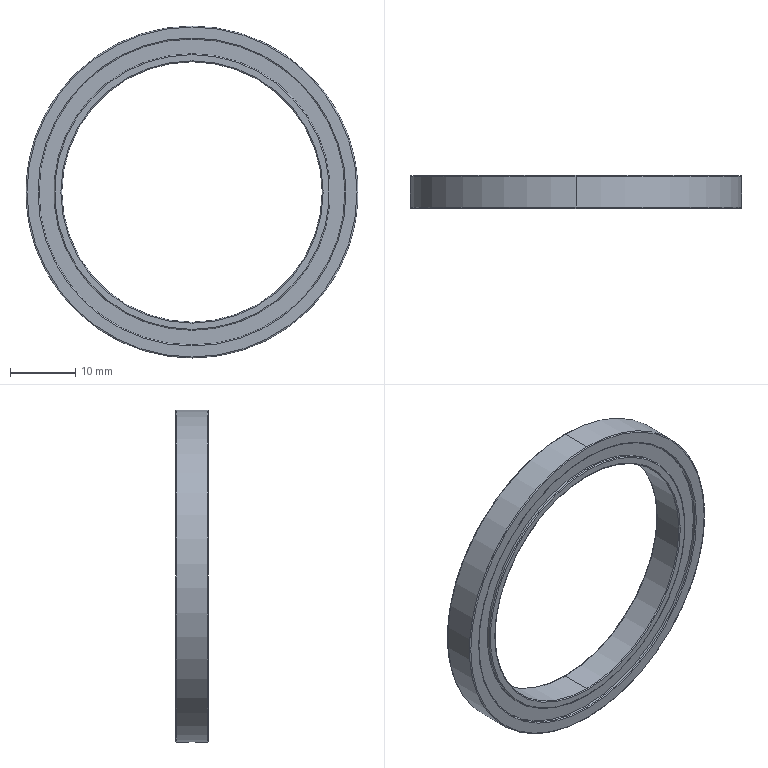Part | SolidWorks | features ICE 3, Extrusion 1, Fillet 1, RefAxis 1, RevCut 1 | 1 solid | 40 faces | box 51 x 5 x 51 mm | volume 3359 mm3 | torus 20 | cylinder 14 | plane 6 | commonest cylinder face diameters 42.5 x4 47 x4 1 x2 40 x2 51 x2
STEP:
#1=CARTESIAN_POINT('',(0.,0.,21.6));
#2=VERTEX_POINT('',#1);
#3=CARTESIAN_POINT('',(0.,0.,23.1));
#4=VERTEX_POINT('',#3);
#5=CARTESIAN_POINT('',(0.,0.,22.35));
#6=DIRECTION('',(-1.,0.,0.));
#7=DIRECTION('',(0.,0.,1.));
#8=AXIS2_PLACEMENT_3D('',#5,#6,#7);
#9=CIRCLE('',#8,0.75);
#10=EDGE_CURVE('',#2,#4,#9,.T.);
#11=ORIENTED_EDGE('',*,*,#10,.T.);
#12=CARTESIAN_POINT('',(0.5,0.,-23.095));
#13=VERTEX_POINT('',#12);
#14=CARTESIAN_POINT('',(0.,0.,0.));
#15=DIRECTION('',(0.,1.,0.));
#16=DIRECTION('',(0.,0.,1.));
#17=AXIS2_PLACEMENT_3D('',#14,#15,#16);
#18=CIRCLE('',#17,23.1);
#19=EDGE_CURVE('',#4,#13,#18,.T.);
#20=ORIENTED_EDGE('',*,*,#19,.T.);
#21=CARTESIAN_POINT('',(0.,-0.5,-22.909));
#22=VERTEX_POINT('',#21);
#23=CARTESIAN_POINT('',(0.5,0.,-23.095));
#24=CARTESIAN_POINT('',(0.5,-0.06758,-23.095));
#25=CARTESIAN_POINT('',(0.4859,-0.1352,-23.085));
#26=CARTESIAN_POINT('',(0.4343,-0.2563,-23.054));
#27=CARTESIAN_POINT('',(0.3972,-0.3102,-23.031));
#28=CARTESIAN_POINT('',(0.3074,-0.3994,-22.985));
#29=CARTESIAN_POINT('',(0.254,-0.4355,-22.96));
#30=CARTESIAN_POINT('',(0.1353,-0.4856,-22.922));
#31=CARTESIAN_POINT('',(0.06827,-0.5,-22.909));
#32=CARTESIAN_POINT('',(0.,-0.5,-22.909));
#33=B_SPLINE_CURVE_WITH_KNOTS('',3,(#23,#24,#25,#26,#27,#28,#29,#30,#31,#32),.UNSPECIFIED.,.F.,.F.,(4,2,2,2,4),(0.002057,0.002259,0.00246,0.002661,0.002863),.UNSPECIFIED.);
#34=EDGE_CURVE('',#13,#22,#33,.T.);
#35=ORIENTED_EDGE('',*,*,#34,.T.);
#36=CARTESIAN_POINT('',(0.,0.,-21.6));
#37=VERTEX_POINT('',#36);
#38=CARTESIAN_POINT('',(0.,0.,-22.35));
#39=DIRECTION('',(1.,0.,0.));
#40=DIRECTION('',(0.,0.,-1.));
#41=AXIS2_PLACEMENT_3D('',#38,#39,#40);
#42=CIRCLE('',#41,0.75);
#43=EDGE_CURVE('',#37,#22,#42,.T.);
#44=ORIENTED_EDGE('',*,*,#43,.F.);
#45=CARTESIAN_POINT('',(0.,0.,0.));
#46=DIRECTION('',(0.,1.,0.));
#47=DIRECTION('',(0.,0.,1.));
#48=AXIS2_PLACEMENT_3D('',#45,#46,#47);
#49=CIRCLE('',#48,21.6);
#50=EDGE_CURVE('',#2,#37,#49,.T.);
#51=ORIENTED_EDGE('',*,*,#50,.F.);
#52=EDGE_LOOP('',(#11,#20,#35,#44,#51));
#53=FACE_OUTER_BOUND('',#52,.T.);
#54=CARTESIAN_POINT('',(0.,0.,0.));
#55=DIRECTION('',(0.,1.,0.));
#56=DIRECTION('',(0.,0.,1.));
#57=AXIS2_PLACEMENT_3D('',#54,#55,#56);
#58=TOROIDAL_SURFACE('',#57,22.35,0.75);
#59=ADVANCED_FACE('',(#53),#58,.F.);
#60=CARTESIAN_POINT('',(-0.5,0.,-23.095));
#61=VERTEX_POINT('',#60);
#62=CARTESIAN_POINT('',(0.,-0.5,-22.909));
#63=CARTESIAN_POINT('',(-0.1367,-0.5,-22.909));
#64=CARTESIAN_POINT('',(-0.2637,-0.4433,-22.962));
#65=CARTESIAN_POINT('',(-0.3982,-0.309,-23.032));
#66=CARTESIAN_POINT('',(-0.4351,-0.2549,-23.054));
#67=CARTESIAN_POINT('',(-0.4859,-0.1348,-23.085));
#68=CARTESIAN_POINT('',(-0.5,-0.06715,-23.095));
#69=CARTESIAN_POINT('',(-0.5,0.,-23.095));
#70=B_SPLINE_CURVE_WITH_KNOTS('',3,(#62,#63,#64,#65,#66,#67,#68,#69),.UNSPECIFIED.,.F.,.F.,(4,2,2,4),(0.002863,0.003266,0.003468,0.003669),.UNSPECIFIED.);
#71=EDGE_CURVE('',#22,#61,#70,.T.);
#72=ORIENTED_EDGE('',*,*,#71,.T.);
#73=CARTESIAN_POINT('',(0.,0.,0.));
#74=DIRECTION('',(0.,1.,0.));
#75=DIRECTION('',(0.,0.,1.));
#76=AXIS2_PLACEMENT_3D('',#73,#74,#75);
#77=CIRCLE('',#76,23.1);
#78=EDGE_CURVE('',#61,#4,#77,.T.);
#79=ORIENTED_EDGE('',*,*,#78,.T.);
#80=ORIENTED_EDGE('',*,*,#10,.F.);
#81=CARTESIAN_POINT('',(0.,0.,0.));
#82=DIRECTION('',(0.,1.,0.));
#83=DIRECTION('',(0.,0.,1.));
#84=AXIS2_PLACEMENT_3D('',#81,#82,#83);
#85=CIRCLE('',#84,21.6);
#86=EDGE_CURVE('',#37,#2,#85,.T.);
#87=ORIENTED_EDGE('',*,*,#86,.F.);
#88=ORIENTED_EDGE('',*,*,#43,.T.);
#89=EDGE_LOOP('',(#72,#79,#80,#87,#88));
#90=FACE_OUTER_BOUND('',#89,.T.);
#91=CARTESIAN_POINT('',(0.,0.,0.));
#92=DIRECTION('',(0.,1.,0.));
#93=DIRECTION('',(0.,0.,1.));
#94=AXIS2_PLACEMENT_3D('',#91,#92,#93);
#95=TOROIDAL_SURFACE('',#94,22.35,0.75);
#96=ADVANCED_FACE('',(#90),#95,.F.);
#97=CARTESIAN_POINT('',(0.,2.5,-23.65));
#98=VERTEX_POINT('',#97);
#99=CARTESIAN_POINT('',(0.,2.5,23.65));
#100=VERTEX_POINT('',#99);
#101=CARTESIAN_POINT('',(0.,2.5,0.));
#102=DIRECTION('',(0.,-1.,0.));
#103=DIRECTION('',(0.,0.,1.));
#104=AXIS2_PLACEMENT_3D('',#101,#102,#103);
#105=CIRCLE('',#104,23.65);
#106=EDGE_CURVE('',#98,#100,#105,.T.);
#107=ORIENTED_EDGE('',*,*,#106,.F.);
#108=CARTESIAN_POINT('',(0.,2.35,-23.5));
#109=VERTEX_POINT('',#108);
#110=CARTESIAN_POINT('',(0.,2.35,-23.65));
#111=DIRECTION('',(1.,0.,0.));
#112=DIRECTION('',(0.,0.,-1.));
#113=AXIS2_PLACEMENT_3D('',#110,#111,#112);
#114=CIRCLE('',#113,0.15);
#115=EDGE_CURVE('',#98,#109,#114,.T.);
#116=ORIENTED_EDGE('',*,*,#115,.T.);
#117=CARTESIAN_POINT('',(0.,2.35,23.5));
#118=VERTEX_POINT('',#117);
#119=CARTESIAN_POINT('',(0.,2.35,0.));
#120=DIRECTION('',(0.,1.,0.));
#121=DIRECTION('',(0.,0.,1.));
#122=AXIS2_PLACEMENT_3D('',#119,#120,#121);
#123=CIRCLE('',#122,23.5);
#124=EDGE_CURVE('',#118,#109,#123,.T.);
#125=ORIENTED_EDGE('',*,*,#124,.F.);
#126=CARTESIAN_POINT('',(0.,2.35,23.65));
#127=DIRECTION('',(-1.,0.,0.));
#128=DIRECTION('',(0.,0.,1.));
#129=AXIS2_PLACEMENT_3D('',#126,#127,#128);
#130=CIRCLE('',#129,0.15);
#131=EDGE_CURVE('',#100,#118,#130,.T.);
#132=ORIENTED_EDGE('',*,*,#131,.F.);
#133=EDGE_LOOP('',(#107,#116,#125,#132));
#134=FACE_OUTER_BOUND('',#133,.T.);
#135=CARTESIAN_POINT('',(0.,2.35,0.));
#136=DIRECTION('',(0.,1.,0.));
#137=DIRECTION('',(0.,0.,1.));
#138=AXIS2_PLACEMENT_3D('',#135,#136,#137);
#139=TOROIDAL_SURFACE('',#138,23.65,0.15);
#140=ADVANCED_FACE('',(#134),#139,.T.);
#141=CARTESIAN_POINT('',(0.,2.35,-25.5));
#142=VERTEX_POINT('',#141);
#143=CARTESIAN_POINT('',(0.,2.35,25.5));
#144=VERTEX_POINT('',#143);
#145=CARTESIAN_POINT('',(0.,2.35,0.));
#146=DIRECTION('',(0.,-1.,0.));
#147=DIRECTION('',(0.,0.,1.));
#148=AXIS2_PLACEMENT_3D('',#145,#146,#147);
#149=CIRCLE('',#148,25.5);
#150=EDGE_CURVE('',#142,#144,#149,.T.);
#151=ORIENTED_EDGE('',*,*,#150,.F.);
#152=CARTESIAN_POINT('',(0.,2.5,-25.35));
#153=VERTEX_POINT('',#152);
#154=CARTESIAN_POINT('',(0.,2.35,-25.35));
#155=DIRECTION('',(1.,0.,0.));
#156=DIRECTION('',(0.,0.,-1.));
#157=AXIS2_PLACEMENT_3D('',#154,#155,#156);
#158=CIRCLE('',#157,0.15);
#159=EDGE_CURVE('',#142,#153,#158,.T.);
#160=ORIENTED_EDGE('',*,*,#159,.T.);
#161=CARTESIAN_POINT('',(0.,2.5,25.35));
#162=VERTEX_POINT('',#161);
#163=CARTESIAN_POINT('',(0.,2.5,0.));
#164=DIRECTION('',(0.,1.,0.));
#165=DIRECTION('',(0.,0.,1.));
#166=AXIS2_PLACEMENT_3D('',#163,#164,#165);
#167=CIRCLE('',#166,25.35);
#168=EDGE_CURVE('',#162,#153,#167,.T.);
#169=ORIENTED_EDGE('',*,*,#168,.F.);
#170=CARTESIAN_POINT('',(0.,2.35,25.35));
#171=DIRECTION('',(-1.,0.,0.));
#172=DIRECTION('',(0.,0.,1.));
#173=AXIS2_PLACEMENT_3D('',#170,#171,#172);
#174=CIRCLE('',#173,0.15);
#175=EDGE_CURVE('',#144,#162,#174,.T.);
#176=ORIENTED_EDGE('',*,*,#175,.F.);
#177=EDGE_LOOP('',(#151,#160,#169,#176));
#178=FACE_OUTER_BOUND('',#177,.T.);
#179=CARTESIAN_POINT('',(0.,2.35,0.));
#180=DIRECTION('',(0.,1.,0.));
#181=DIRECTION('',(0.,0.,1.));
#182=AXIS2_PLACEMENT_3D('',#179,#180,#181);
#183=TOROIDAL_SURFACE('',#182,25.35,0.15);
#184=ADVANCED_FACE('',(#178),#183,.T.);
#185=CARTESIAN_POINT('',(0.,2.5,-20.15));
#186=VERTEX_POINT('',#185);
#187=CARTESIAN_POINT('',(0.,2.5,20.15));
#188=VERTEX_POINT('',#187);
#189=CARTESIAN_POINT('',(0.,2.5,0.));
#190=DIRECTION('',(0.,-1.,0.));
#191=DIRECTION('',(0.,0.,1.));
#192=AXIS2_PLACEMENT_3D('',#189,#190,#191);
#193=CIRCLE('',#192,20.15);
#194=EDGE_CURVE('',#186,#188,#193,.T.);
#195=ORIENTED_EDGE('',*,*,#194,.F.);
#196=CARTESIAN_POINT('',(0.,2.35,-20.));
#197=VERTEX_POINT('',#196);
#198=CARTESIAN_POINT('',(0.,2.35,-20.15));
#199=DIRECTION('',(1.,0.,0.));
#200=DIRECTION('',(0.,0.,-1.));
#201=AXIS2_PLACEMENT_3D('',#198,#199,#200);
#202=CIRCLE('',#201,0.15);
#203=EDGE_CURVE('',#186,#197,#202,.T.);
#204=ORIENTED_EDGE('',*,*,#203,.T.);
#205=CARTESIAN_POINT('',(0.,2.35,20.));
#206=VERTEX_POINT('',#205);
#207=CARTESIAN_POINT('',(0.,2.35,0.));
#208=DIRECTION('',(0.,1.,0.));
#209=DIRECTION('',(0.,0.,1.));
#210=AXIS2_PLACEMENT_3D('',#207,#208,#209);
#211=CIRCLE('',#210,20.);
#212=EDGE_CURVE('',#206,#197,#211,.T.);
#213=ORIENTED_EDGE('',*,*,#212,.F.);
#214=CARTESIAN_POINT('',(0.,2.35,20.15));
#215=DIRECTION('',(-1.,0.,0.));
#216=DIRECTION('',(0.,0.,1.));
#217=AXIS2_PLACEMENT_3D('',#214,#215,#216);
#218=CIRCLE('',#217,0.15);
#219=EDGE_CURVE('',#188,#206,#218,.T.);
#220=ORIENTED_EDGE('',*,*,#219,.F.);
#221=EDGE_LOOP('',(#195,#204,#213,#220));
#222=FACE_OUTER_BOUND('',#221,.T.);
#223=CARTESIAN_POINT('',(0.,2.35,0.));
#224=DIRECTION('',(0.,1.,0.));
#225=DIRECTION('',(0.,0.,1.));
#226=AXIS2_PLACEMENT_3D('',#223,#224,#225);
#227=TOROIDAL_SURFACE('',#226,20.15,0.15);
#228=ADVANCED_FACE('',(#222),#227,.T.);
#229=CARTESIAN_POINT('',(0.,2.35,-21.25));
#230=VERTEX_POINT('',#229);
#231=CARTESIAN_POINT('',(0.,2.35,21.25));
#232=VERTEX_POINT('',#231);
#233=CARTESIAN_POINT('',(0.,2.35,0.));
#234=DIRECTION('',(0.,-1.,0.));
#235=DIRECTION('',(0.,0.,1.));
#236=AXIS2_PLACEMENT_3D('',#233,#234,#235);
#237=CIRCLE('',#236,21.25);
#238=EDGE_CURVE('',#230,#232,#237,.T.);
#239=ORIENTED_EDGE('',*,*,#238,.F.);
#240=CARTESIAN_POINT('',(0.,2.5,-21.1));
#241=VERTEX_POINT('',#240);
#242=CARTESIAN_POINT('',(0.,2.35,-21.1));
#243=DIRECTION('',(1.,0.,0.));
#244=DIRECTION('',(0.,0.,-1.));
#245=AXIS2_PLACEMENT_3D('',#242,#243,#244);
#246=CIRCLE('',#245,0.15);
#247=EDGE_CURVE('',#230,#241,#246,.T.);
#248=ORIENTED_EDGE('',*,*,#247,.T.);
#249=CARTESIAN_POINT('',(0.,2.5,21.1));
#250=VERTEX_POINT('',#249);
#251=CARTESIAN_POINT('',(0.,2.5,0.));
#252=DIRECTION('',(0.,1.,0.));
#253=DIRECTION('',(0.,0.,1.));
#254=AXIS2_PLACEMENT_3D('',#251,#252,#253);
#255=CIRCLE('',#254,21.1);
#256=EDGE_CURVE('',#250,#241,#255,.T.);
#257=ORIENTED_EDGE('',*,*,#256,.F.);
#258=CARTESIAN_POINT('',(0.,2.35,21.1));
#259=DIRECTION('',(-1.,0.,0.));
#260=DIRECTION('',(0.,0.,1.));
#261=AXIS2_PLACEMENT_3D('',#258,#259,#260);
#262=CIRCLE('',#261,0.15);
#263=EDGE_CURVE('',#232,#250,#262,.T.);
#264=ORIENTED_EDGE('',*,*,#263,.F.);
#265=EDGE_LOOP('',(#239,#248,#257,#264));
#266=FACE_OUTER_BOUND('',#265,.T.);
#267=CARTESIAN_POINT('',(0.,2.35,0.));
#268=DIRECTION('',(0.,1.,0.));
#269=DIRECTION('',(0.,0.,1.));
#270=AXIS2_PLACEMENT_3D('',#267,#268,#269);
#271=TOROIDAL_SURFACE('',#270,21.1,0.15);
#272=ADVANCED_FACE('',(#266),#271,.T.);
#273=CARTESIAN_POINT('',(0.,-2.35,-23.5));
#274=VERTEX_POINT('',#273);
#275=CARTESIAN_POINT('',(0.,-2.35,23.5));
#276=VERTEX_POINT('',#275);
#277=CARTESIAN_POINT('',(0.,-2.35,0.));
#278=DIRECTION('',(0.,-1.,0.));
#279=DIRECTION('',(0.,0.,1.));
#280=AXIS2_PLACEMENT_3D('',#277,#278,#279);
#281=CIRCLE('',#280,23.5);
#282=EDGE_CURVE('',#274,#276,#281,.T.);
#283=ORIENTED_EDGE('',*,*,#282,.F.);
#284=CARTESIAN_POINT('',(0.,-2.5,-23.65));
#285=VERTEX_POINT('',#284);
#286=CARTESIAN_POINT('',(0.,-2.35,-23.65));
#287=DIRECTION('',(1.,0.,0.));
#288=DIRECTION('',(0.,0.,-1.));
#289=AXIS2_PLACEMENT_3D('',#286,#287,#288);
#290=CIRCLE('',#289,0.15);
#291=EDGE_CURVE('',#274,#285,#290,.T.);
#292=ORIENTED_EDGE('',*,*,#291,.T.);
#293=CARTESIAN_POINT('',(0.,-2.5,23.65));
#294=VERTEX_POINT('',#293);
#295=CARTESIAN_POINT('',(0.,-2.5,0.));
#296=DIRECTION('',(0.,1.,0.));
#297=DIRECTION('',(0.,0.,1.));
#298=AXIS2_PLACEMENT_3D('',#295,#296,#297);
#299=CIRCLE('',#298,23.65);
#300=EDGE_CURVE('',#294,#285,#299,.T.);
#301=ORIENTED_EDGE('',*,*,#300,.F.);
#302=CARTESIAN_POINT('',(0.,-2.35,23.65));
#303=DIRECTION('',(-1.,0.,0.));
#304=DIRECTION('',(0.,0.,1.));
#305=AXIS2_PLACEMENT_3D('',#302,#303,#304);
#306=CIRCLE('',#305,0.15);
#307=EDGE_CURVE('',#276,#294,#306,.T.);
#308=ORIENTED_EDGE('',*,*,#307,.F.);
#309=EDGE_LOOP('',(#283,#292,#301,#308));
#310=FACE_OUTER_BOUND('',#309,.T.);
#311=CARTESIAN_POINT('',(0.,-2.35,0.));
#312=DIRECTION('',(0.,1.,0.));
#313=DIRECTION('',(0.,0.,1.));
#314=AXIS2_PLACEMENT_3D('',#311,#312,#313);
#315=TOROIDAL_SURFACE('',#314,23.65,0.15);
#316=ADVANCED_FACE('',(#310),#315,.T.);
#317=CARTESIAN_POINT('',(0.,-2.5,-25.35));
#318=VERTEX_POINT('',#317);
#319=CARTESIAN_POINT('',(0.,-2.5,25.35));
#320=VERTEX_POINT('',#319);
#321=CARTESIAN_POINT('',(0.,-2.5,0.));
#322=DIRECTION('',(0.,-1.,0.));
#323=DIRECTION('',(0.,0.,1.));
#324=AXIS2_PLACEMENT_3D('',#321,#322,#323);
#325=CIRCLE('',#324,25.35);
#326=EDGE_CURVE('',#318,#320,#325,.T.);
#327=ORIENTED_EDGE('',*,*,#326,.F.);
#328=CARTESIAN_POINT('',(0.,-2.35,-25.5));
#329=VERTEX_POINT('',#328);
#330=CARTESIAN_POINT('',(0.,-2.35,-25.35));
#331=DIRECTION('',(1.,0.,0.));
#332=DIRECTION('',(0.,0.,-1.));
#333=AXIS2_PLACEMENT_3D('',#330,#331,#332);
#334=CIRCLE('',#333,0.15);
#335=EDGE_CURVE('',#318,#329,#334,.T.);
#336=ORIENTED_EDGE('',*,*,#335,.T.);
#337=CARTESIAN_POINT('',(0.,-2.35,25.5));
#338=VERTEX_POINT('',#337);
#339=CARTESIAN_POINT('',(0.,-2.35,0.));
#340=DIRECTION('',(0.,1.,0.));
#341=DIRECTION('',(0.,0.,1.));
#342=AXIS2_PLACEMENT_3D('',#339,#340,#341);
#343=CIRCLE('',#342,25.5);
#344=EDGE_CURVE('',#338,#329,#343,.T.);
#345=ORIENTED_EDGE('',*,*,#344,.F.);
#346=CARTESIAN_POINT('',(0.,-2.35,25.35));
#347=DIRECTION('',(-1.,0.,0.));
#348=DIRECTION('',(0.,0.,1.));
#349=AXIS2_PLACEMENT_3D('',#346,#347,#348);
#350=CIRCLE('',#349,0.15);
#351=EDGE_CURVE('',#320,#338,#350,.T.);
#352=ORIENTED_EDGE('',*,*,#351,.F.);
#353=EDGE_LOOP('',(#327,#336,#345,#352));
#354=FACE_OUTER_BOUND('',#353,.T.);
#355=CARTESIAN_POINT('',(0.,-2.35,0.));
#356=DIRECTION('',(0.,1.,0.));
#357=DIRECTION('',(0.,0.,1.));
#358=AXIS2_PLACEMENT_3D('',#355,#356,#357);
#359=TOROIDAL_SURFACE('',#358,25.35,0.15);
#360=ADVANCED_FACE('',(#354),#359,.T.);
#361=CARTESIAN_POINT('',(0.,-2.35,-20.));
#362=VERTEX_POINT('',#361);
#363=CARTESIAN_POINT('',(0.,-2.35,20.));
#364=VERTEX_POINT('',#363);
#365=CARTESIAN_POINT('',(0.,-2.35,0.));
#366=DIRECTION('',(0.,-1.,0.));
#367=DIRECTION('',(0.,0.,1.));
#368=AXIS2_PLACEMENT_3D('',#365,#366,#367);
#369=CIRCLE('',#368,20.);
#370=EDGE_CURVE('',#362,#364,#369,.T.);
#371=ORIENTED_EDGE('',*,*,#370,.F.);
#372=CARTESIAN_POINT('',(0.,-2.5,-20.15));
#373=VERTEX_POINT('',#372);
#374=CARTESIAN_POINT('',(0.,-2.35,-20.15));
#375=DIRECTION('',(1.,0.,0.));
#376=DIRECTION('',(0.,0.,-1.));
#377=AXIS2_PLACEMENT_3D('',#374,#375,#376);
#378=CIRCLE('',#377,0.15);
#379=EDGE_CURVE('',#362,#373,#378,.T.);
#380=ORIENTED_EDGE('',*,*,#379,.T.);
#381=CARTESIAN_POINT('',(0.,-2.5,20.15));
#382=VERTEX_POINT('',#381);
#383=CARTESIAN_POINT('',(0.,-2.5,0.));
#384=DIRECTION('',(0.,1.,0.));
#385=DIRECTION('',(0.,0.,1.));
#386=AXIS2_PLACEMENT_3D('',#383,#384,#385);
#387=CIRCLE('',#386,20.15);
#388=EDGE_CURVE('',#382,#373,#387,.T.);
#389=ORIENTED_EDGE('',*,*,#388,.F.);
#390=CARTESIAN_POINT('',(0.,-2.35,20.15));
#391=DIRECTION('',(-1.,0.,0.));
#392=DIRECTION('',(0.,0.,1.));
#393=AXIS2_PLACEMENT_3D('',#390,#391,#392);
#394=CIRCLE('',#393,0.15);
#395=EDGE_CURVE('',#364,#382,#394,.T.);
#396=ORIENTED_EDGE('',*,*,#395,.F.);
#397=EDGE_LOOP('',(#371,#380,#389,#396));
#398=FACE_OUTER_BOUND('',#397,.T.);
#399=CARTESIAN_POINT('',(0.,-2.35,0.));
#400=DIRECTION('',(0.,1.,0.));
#401=DIRECTION('',(0.,0.,1.));
#402=AXIS2_PLACEMENT_3D('',#399,#400,#401);
#403=TOROIDAL_SURFACE('',#402,20.15,0.15);
#404=ADVANCED_FACE('',(#398),#403,.T.);
#405=CARTESIAN_POINT('',(0.,-2.5,-21.1));
#406=VERTEX_POINT('',#405);
#407=CARTESIAN_POINT('',(0.,-2.5,21.1));
#408=VERTEX_POINT('',#407);
#409=CARTESIAN_POINT('',(0.,-2.5,0.));
#410=DIRECTION('',(0.,-1.,0.));
#411=DIRECTION('',(0.,0.,1.));
#412=AXIS2_PLACEMENT_3D('',#409,#410,#411);
#413=CIRCLE('',#412,21.1);
#414=EDGE_CURVE('',#406,#408,#413,.T.);
#415=ORIENTED_EDGE('',*,*,#414,.F.);
#416=CARTESIAN_POINT('',(0.,-2.35,-21.25));
#417=VERTEX_POINT('',#416);
#418=CARTESIAN_POINT('',(0.,-2.35,-21.1));
#419=DIRECTION('',(1.,0.,0.));
#420=DIRECTION('',(0.,0.,-1.));
#421=AXIS2_PLACEMENT_3D('',#418,#419,#420);
#422=CIRCLE('',#421,0.15);
#423=EDGE_CURVE('',#406,#417,#422,.T.);
#424=ORIENTED_EDGE('',*,*,#423,.T.);
#425=CARTESIAN_POINT('',(0.,-2.35,21.25));
#426=VERTEX_POINT('',#425);
#427=CARTESIAN_POINT('',(0.,-2.35,0.));
#428=DIRECTION('',(0.,1.,0.));
#429=DIRECTION('',(0.,0.,1.));
#430=AXIS2_PLACEMENT_3D('',#427,#428,#429);
#431=CIRCLE('',#430,21.25);
#432=EDGE_CURVE('',#426,#417,#431,.T.);
#433=ORIENTED_EDGE('',*,*,#432,.F.);
#434=CARTESIAN_POINT('',(0.,-2.35,21.1));
#435=DIRECTION('',(-1.,0.,0.));
#436=DIRECTION('',(0.,0.,1.));
#437=AXIS2_PLACEMENT_3D('',#434,#435,#436);
#438=CIRCLE('',#437,0.15);
#439=EDGE_CURVE('',#408,#426,#438,.T.);
#440=ORIENTED_EDGE('',*,*,#439,.F.);
#441=EDGE_LOOP('',(#415,#424,#433,#440));
#442=FACE_OUTER_BOUND('',#441,.T.);
#443=CARTESIAN_POINT('',(0.,-2.35,0.));
#444=DIRECTION('',(0.,1.,0.));
#445=DIRECTION('',(0.,0.,1.));
#446=AXIS2_PLACEMENT_3D('',#443,#444,#445);
#447=TOROIDAL_SURFACE('',#446,21.1,0.15);
#448=ADVANCED_FACE('',(#442),#447,.T.);
#449=ORIENTED_EDGE('',*,*,#78,.F.);
#450=CARTESIAN_POINT('',(0.,0.5,-22.909));
#451=VERTEX_POINT('',#450);
#452=CARTESIAN_POINT('',(-0.5,0.,-23.095));
#453=CARTESIAN_POINT('',(-0.5,0.06713,-23.095));
#454=CARTESIAN_POINT('',(-0.4861,0.1346,-23.085));
#455=CARTESIAN_POINT('',(-0.4343,0.2564,-23.054));
#456=CARTESIAN_POINT('',(-0.3973,0.3101,-23.031));
#457=CARTESIAN_POINT('',(-0.2623,0.4441,-22.961));
#458=CARTESIAN_POINT('',(-0.136,0.5,-22.909));
#459=CARTESIAN_POINT('',(0.,0.5,-22.909));
#460=B_SPLINE_CURVE_WITH_KNOTS('',3,(#452,#453,#454,#455,#456,#457,#458,#459),.UNSPECIFIED.,.F.,.F.,(4,2,2,4),(0.0004431,0.0006447,0.0008463,0.00125),.UNSPECIFIED.);
#461=EDGE_CURVE('',#61,#451,#460,.T.);
#462=ORIENTED_EDGE('',*,*,#461,.T.);
#463=CARTESIAN_POINT('',(0.,0.,-22.35));
#464=DIRECTION('',(1.,0.,0.));
#465=DIRECTION('',(0.,0.,-1.));
#466=AXIS2_PLACEMENT_3D('',#463,#464,#465);
#467=CIRCLE('',#466,0.75);
#468=EDGE_CURVE('',#451,#37,#467,.T.);
#469=ORIENTED_EDGE('',*,*,#468,.T.);
#470=ORIENTED_EDGE('',*,*,#86,.T.);
#471=CARTESIAN_POINT('',(0.,0.,22.35));
#472=DIRECTION('',(-1.,0.,0.));
#473=DIRECTION('',(0.,0.,1.));
#474=AXIS2_PLACEMENT_3D('',#471,#472,#473);
#475=CIRCLE('',#474,0.75);
#476=EDGE_CURVE('',#4,#2,#475,.T.);
#477=ORIENTED_EDGE('',*,*,#476,.F.);
#478=EDGE_LOOP('',(#449,#462,#469,#470,#477));
#479=FACE_OUTER_BOUND('',#478,.T.);
#480=CARTESIAN_POINT('',(0.,0.,0.));
#481=DIRECTION('',(0.,1.,0.));
#482=DIRECTION('',(0.,0.,1.));
#483=AXIS2_PLACEMENT_3D('',#480,#481,#482);
#484=TOROIDAL_SURFACE('',#483,22.35,0.75);
#485=ADVANCED_FACE('',(#479),#484,.F.);
#486=CARTESIAN_POINT('',(-0.5,-0.00007979,-25.495));
#487=VERTEX_POINT('',#486);
#488=CARTESIAN_POINT('',(0.,-0.5,-25.5));
#489=VERTEX_POINT('',#488);
#490=CARTESIAN_POINT('',(-0.5,-0.00007979,-25.495));
#491=CARTESIAN_POINT('',(-0.5,-0.1381,-25.495));
#492=CARTESIAN_POINT('',(-0.4512,-0.2559,-25.496));
#493=CARTESIAN_POINT('',(-0.2559,-0.4512,-25.499));
#494=CARTESIAN_POINT('',(-0.1381,-0.5,-25.5));
#495=CARTESIAN_POINT('',(0.,-0.5,-25.5));
#496=B_SPLINE_CURVE_WITH_KNOTS('',3,(#490,#491,#492,#493,#494,#495),.UNSPECIFIED.,.F.,.F.,(4,2,4),(0.5002,0.7501,1.),.UNSPECIFIED.);
#497=EDGE_CURVE('',#487,#489,#496,.T.);
#498=ORIENTED_EDGE('',*,*,#497,.F.);
#499=CARTESIAN_POINT('',(-0.5,0.,-25.5));
#500=DIRECTION('',(0.,0.,1.));
#501=VECTOR('',#500,1000.);
#502=LINE('',#499,#501);
#503=EDGE_CURVE('',#487,#61,#502,.T.);
#504=ORIENTED_EDGE('',*,*,#503,.T.);
#505=ORIENTED_EDGE('',*,*,#71,.F.);
#506=ORIENTED_EDGE('',*,*,#34,.F.);
#507=CARTESIAN_POINT('',(0.5,-0.000002672,-25.495));
#508=VERTEX_POINT('',#507);
#509=CARTESIAN_POINT('',(0.5,0.,-25.5));
#510=DIRECTION('',(0.,0.,1.));
#511=VECTOR('',#510,1000.);
#512=LINE('',#509,#511);
#513=EDGE_CURVE('',#508,#13,#512,.T.);
#514=ORIENTED_EDGE('',*,*,#513,.F.);
#515=CARTESIAN_POINT('',(0.,-0.5,-25.5));
#516=CARTESIAN_POINT('',(0.138,-0.5,-25.5));
#517=CARTESIAN_POINT('',(0.2558,-0.4513,-25.499));
#518=CARTESIAN_POINT('',(0.4511,-0.256,-25.496));
#519=CARTESIAN_POINT('',(0.5,-0.1381,-25.495));
#520=CARTESIAN_POINT('',(0.5,-0.000002672,-25.495));
#521=B_SPLINE_CURVE_WITH_KNOTS('',3,(#515,#516,#517,#518,#519,#520),.UNSPECIFIED.,.F.,.F.,(4,2,4),(0.,0.2501,0.5003),.UNSPECIFIED.);
#522=EDGE_CURVE('',#489,#508,#521,.T.);
#523=ORIENTED_EDGE('',*,*,#522,.F.);
#524=EDGE_LOOP('',(#498,#504,#505,#506,#514,#523));
#525=FACE_OUTER_BOUND('',#524,.T.);
#526=CARTESIAN_POINT('',(0.,0.,-25.5));
#527=DIRECTION('',(0.,0.,1.));
#528=DIRECTION('',(1.,0.,0.));
#529=AXIS2_PLACEMENT_3D('',#526,#527,#528);
#530=CYLINDRICAL_SURFACE('',#529,0.5);
#531=ADVANCED_FACE('',(#525),#530,.F.);
#532=CARTESIAN_POINT('',(0.,-2.,-21.25));
#533=VERTEX_POINT('',#532);
#534=CARTESIAN_POINT('',(0.,-2.,21.25));
#535=VERTEX_POINT('',#534);
#536=CARTESIAN_POINT('',(0.,-2.,0.));
#537=DIRECTION('',(0.,-1.,0.));
#538=DIRECTION('',(0.,0.,-1.));
#539=AXIS2_PLACEMENT_3D('',#536,#537,#538);
#540=CIRCLE('',#539,21.25);
#541=EDGE_CURVE('',#533,#535,#540,.T.);
#542=ORIENTED_EDGE('',*,*,#541,.T.);
#543=CARTESIAN_POINT('',(0.,-2.,21.25));
#544=DIRECTION('',(0.,-1.,0.));
#545=VECTOR('',#544,1000.);
#546=LINE('',#543,#545);
#547=EDGE_CURVE('',#535,#426,#546,.T.);
#548=ORIENTED_EDGE('',*,*,#547,.T.);
#549=ORIENTED_EDGE('',*,*,#432,.T.);
#550=CARTESIAN_POINT('',(0.,-2.,-21.25));
#551=DIRECTION('',(0.,-1.,0.));
#552=VECTOR('',#551,1000.);
#553=LINE('',#550,#552);
#554=EDGE_CURVE('',#533,#417,#553,.T.);
#555=ORIENTED_EDGE('',*,*,#554,.F.);
#556=EDGE_LOOP('',(#542,#548,#549,#555));
#557=FACE_OUTER_BOUND('',#556,.T.);
#558=CARTESIAN_POINT('',(0.,-2.,0.));
#559=DIRECTION('',(0.,-1.,0.));
#560=DIRECTION('',(0.,0.,-1.));
#561=AXIS2_PLACEMENT_3D('',#558,#559,#560);
#562=CYLINDRICAL_SURFACE('',#561,21.25);
#563=ADVANCED_FACE('',(#557),#562,.T.);
#564=CARTESIAN_POINT('',(0.,-2.,23.5));
#565=VERTEX_POINT('',#564);
#566=CARTESIAN_POINT('',(0.,-2.,-23.5));
#567=VERTEX_POINT('',#566);
#568=CARTESIAN_POINT('',(0.,-2.,0.));
#569=DIRECTION('',(0.,-1.,0.));
#570=DIRECTION('',(0.,0.,-1.));
#571=AXIS2_PLACEMENT_3D('',#568,#569,#570);
#572=CIRCLE('',#571,23.5);
#573=EDGE_CURVE('',#565,#567,#572,.T.);
#574=ORIENTED_EDGE('',*,*,#573,.F.);
#575=CARTESIAN_POINT('',(0.,-2.,23.5));
#576=DIRECTION('',(0.,-1.,0.));
#577=VECTOR('',#576,1000.);
#578=LINE('',#575,#577);
#579=EDGE_CURVE('',#565,#276,#578,.T.);
#580=ORIENTED_EDGE('',*,*,#579,.T.);
#581=CARTESIAN_POINT('',(0.,-2.35,0.));
#582=DIRECTION('',(0.,-1.,0.));
#583=DIRECTION('',(0.,0.,1.));
#584=AXIS2_PLACEMENT_3D('',#581,#582,#583);
#585=CIRCLE('',#584,23.5);
#586=EDGE_CURVE('',#276,#274,#585,.T.);
#587=ORIENTED_EDGE('',*,*,#586,.T.);
#588=CARTESIAN_POINT('',(0.,-2.,-23.5));
#589=DIRECTION('',(0.,-1.,0.));
#590=VECTOR('',#589,1000.);
#591=LINE('',#588,#590);
#592=EDGE_CURVE('',#567,#274,#591,.T.);
#593=ORIENTED_EDGE('',*,*,#592,.F.);
#594=EDGE_LOOP('',(#574,#580,#587,#593));
#595=FACE_OUTER_BOUND('',#594,.T.);
#596=CARTESIAN_POINT('',(0.,-2.,0.));
#597=DIRECTION('',(0.,-1.,0.));
#598=DIRECTION('',(0.,0.,-1.));
#599=AXIS2_PLACEMENT_3D('',#596,#597,#598);
#600=CYLINDRICAL_SURFACE('',#599,23.5);
#601=ADVANCED_FACE('',(#595),#600,.F.);
#602=CARTESIAN_POINT('',(0.,2.,21.25));
#603=VERTEX_POINT('',#602);
#604=CARTESIAN_POINT('',(0.,2.,-21.25));
#605=VERTEX_POINT('',#604);
#606=CARTESIAN_POINT('',(0.,2.,0.));
#607=DIRECTION('',(0.,1.,0.));
#608=DIRECTION('',(0.,0.,1.));
#609=AXIS2_PLACEMENT_3D('',#606,#607,#608);
#610=CIRCLE('',#609,21.25);
#611=EDGE_CURVE('',#603,#605,#610,.T.);
#612=ORIENTED_EDGE('',*,*,#611,.T.);
#613=CARTESIAN_POINT('',(0.,2.,-21.25));
#614=DIRECTION('',(0.,1.,0.));
#615=VECTOR('',#614,1000.);
#616=LINE('',#613,#615);
#617=EDGE_CURVE('',#605,#230,#616,.T.);
#618=ORIENTED_EDGE('',*,*,#617,.T.);
#619=ORIENTED_EDGE('',*,*,#238,.T.);
#620=CARTESIAN_POINT('',(0.,2.,21.25));
#621=DIRECTION('',(0.,1.,0.));
#622=VECTOR('',#621,1000.);
#623=LINE('',#620,#622);
#624=EDGE_CURVE('',#603,#232,#623,.T.);
#625=ORIENTED_EDGE('',*,*,#624,.F.);
#626=EDGE_LOOP('',(#612,#618,#619,#625));
#627=FACE_OUTER_BOUND('',#626,.T.);
#628=CARTESIAN_POINT('',(0.,2.,0.));
#629=DIRECTION('',(0.,1.,0.));
#630=DIRECTION('',(0.,0.,1.));
#631=AXIS2_PLACEMENT_3D('',#628,#629,#630);
#632=CYLINDRICAL_SURFACE('',#631,21.25);
#633=ADVANCED_FACE('',(#627),#632,.T.);
#634=CARTESIAN_POINT('',(0.,2.,-23.5));
#635=VERTEX_POINT('',#634);
#636=CARTESIAN_POINT('',(0.,2.,23.5));
#637=VERTEX_POINT('',#636);
#638=CARTESIAN_POINT('',(0.,2.,0.));
#639=DIRECTION('',(0.,1.,0.));
#640=DIRECTION('',(0.,0.,1.));
#641=AXIS2_PLACEMENT_3D('',#638,#639,#640);
#642=CIRCLE('',#641,23.5);
#643=EDGE_CURVE('',#635,#637,#642,.T.);
#644=ORIENTED_EDGE('',*,*,#643,.F.);
#645=CARTESIAN_POINT('',(0.,2.,-23.5));
#646=DIRECTION('',(0.,1.,0.));
#647=VECTOR('',#646,1000.);
#648=LINE('',#645,#647);
#649=EDGE_CURVE('',#635,#109,#648,.T.);
#650=ORIENTED_EDGE('',*,*,#649,.T.);
#651=CARTESIAN_POINT('',(0.,2.35,0.));
#652=DIRECTION('',(0.,1.,0.));
#653=DIRECTION('',(0.,0.,1.));
#654=AXIS2_PLACEMENT_3D('',#651,#652,#653);
#655=CIRCLE('',#654,23.5);
#656=EDGE_CURVE('',#109,#118,#655,.T.);
#657=ORIENTED_EDGE('',*,*,#656,.T.);
#658=CARTESIAN_POINT('',(0.,2.,23.5));
#659=DIRECTION('',(0.,1.,0.));
#660=VECTOR('',#659,1000.);
#661=LINE('',#658,#660);
#662=EDGE_CURVE('',#637,#118,#661,.T.);
#663=ORIENTED_EDGE('',*,*,#662,.F.);
#664=EDGE_LOOP('',(#644,#650,#657,#663));
#665=FACE_OUTER_BOUND('',#664,.T.);
#666=CARTESIAN_POINT('',(0.,2.,0.));
#667=DIRECTION('',(0.,1.,0.));
#668=DIRECTION('',(0.,0.,1.));
#669=AXIS2_PLACEMENT_3D('',#666,#667,#668);
#670=CYLINDRICAL_SURFACE('',#669,23.5);
#671=ADVANCED_FACE('',(#665),#670,.F.);
#672=CARTESIAN_POINT('',(0.,2.35,0.));
#673=DIRECTION('',(0.,1.,0.));
#674=DIRECTION('',(0.,0.,1.));
#675=AXIS2_PLACEMENT_3D('',#672,#673,#674);
#676=CIRCLE('',#675,20.);
#677=EDGE_CURVE('',#197,#206,#676,.T.);
#678=ORIENTED_EDGE('',*,*,#677,.T.);
#679=CARTESIAN_POINT('',(0.,2.5,20.));
#680=DIRECTION('',(0.,-1.,0.));
#681=VECTOR('',#680,1000.);
#682=LINE('',#679,#681);
#683=EDGE_CURVE('',#206,#364,#682,.T.);
#684=ORIENTED_EDGE('',*,*,#683,.T.);
#685=CARTESIAN_POINT('',(0.,-2.35,0.));
#686=DIRECTION('',(0.,-1.,0.));
#687=DIRECTION('',(0.,0.,1.));
#688=AXIS2_PLACEMENT_3D('',#685,#686,#687);
#689=CIRCLE('',#688,20.);
#690=EDGE_CURVE('',#364,#362,#689,.T.);
#691=ORIENTED_EDGE('',*,*,#690,.T.);
#692=CARTESIAN_POINT('',(0.,2.5,-20.));
#693=DIRECTION('',(0.,-1.,0.));
#694=VECTOR('',#693,1000.);
#695=LINE('',#692,#694);
#696=EDGE_CURVE('',#197,#362,#695,.T.);
#697=ORIENTED_EDGE('',*,*,#696,.F.);
#698=EDGE_LOOP('',(#678,#684,#691,#697));
#699=FACE_OUTER_BOUND('',#698,.T.);
#700=CARTESIAN_POINT('',(0.,2.5,0.));
#701=DIRECTION('',(0.,-1.,0.));
#702=DIRECTION('',(0.,0.,-1.));
#703=AXIS2_PLACEMENT_3D('',#700,#701,#702);
#704=CYLINDRICAL_SURFACE('',#703,20.);
#705=ADVANCED_FACE('',(#699),#704,.F.);
#706=ORIENTED_EDGE('',*,*,#150,.T.);
#707=CARTESIAN_POINT('',(0.,2.5,25.5));
#708=DIRECTION('',(0.,-1.,0.));
#709=VECTOR('',#708,1000.);
#710=LINE('',#707,#709);
#711=EDGE_CURVE('',#144,#338,#710,.T.);
#712=ORIENTED_EDGE('',*,*,#711,.T.);
#713=ORIENTED_EDGE('',*,*,#344,.T.);
#714=CARTESIAN_POINT('',(0.,2.5,-25.5));
#715=DIRECTION('',(0.,-1.,0.));
#716=VECTOR('',#715,1000.);
#717=LINE('',#714,#716);
#718=EDGE_CURVE('',#489,#329,#717,.T.);
#719=ORIENTED_EDGE('',*,*,#718,.F.);
#720=ORIENTED_EDGE('',*,*,#522,.T.);
#721=CARTESIAN_POINT('',(0.,0.5,-25.5));
#722=VERTEX_POINT('',#721);
#723=CARTESIAN_POINT('',(0.5,-0.000002672,-25.495));
#724=CARTESIAN_POINT('',(0.5,0.138,-25.495));
#725=CARTESIAN_POINT('',(0.4513,0.2558,-25.496));
#726=CARTESIAN_POINT('',(0.256,0.4512,-25.499));
#727=CARTESIAN_POINT('',(0.1381,0.5,-25.5));
#728=CARTESIAN_POINT('',(0.,0.5,-25.5));
#729=B_SPLINE_CURVE_WITH_KNOTS('',3,(#723,#724,#725,#726,#727,#728),.UNSPECIFIED.,.F.,.F.,(4,2,4),(0.5003,0.7501,1.),.UNSPECIFIED.);
#730=EDGE_CURVE('',#508,#722,#729,.T.);
#731=ORIENTED_EDGE('',*,*,#730,.T.);
#732=CARTESIAN_POINT('',(0.,2.5,-25.5));
#733=DIRECTION('',(0.,-1.,0.));
#734=VECTOR('',#733,1000.);
#735=LINE('',#732,#734);
#736=EDGE_CURVE('',#142,#722,#735,.T.);
#737=ORIENTED_EDGE('',*,*,#736,.F.);
#738=EDGE_LOOP('',(#706,#712,#713,#719,#720,#731,#737));
#739=FACE_OUTER_BOUND('',#738,.T.);
#740=CARTESIAN_POINT('',(0.,2.5,0.));
#741=DIRECTION('',(0.,-1.,0.));
#742=DIRECTION('',(0.,0.,-1.));
#743=AXIS2_PLACEMENT_3D('',#740,#741,#742);
#744=CYLINDRICAL_SURFACE('',#743,25.5);
#745=ADVANCED_FACE('',(#739),#744,.T.);
#746=CARTESIAN_POINT('',(0.,-2.5,0.));
#747=DIRECTION('',(0.,-1.,0.));
#748=DIRECTION('',(0.,0.,1.));
#749=AXIS2_PLACEMENT_3D('',#746,#747,#748);
#750=CIRCLE('',#749,21.1);
#751=EDGE_CURVE('',#408,#406,#750,.T.);
#752=ORIENTED_EDGE('',*,*,#751,.T.);
#753=ORIENTED_EDGE('',*,*,#414,.T.);
#754=EDGE_LOOP('',(#752,#753));
#755=FACE_OUTER_BOUND('',#754,.T.);
#756=ORIENTED_EDGE('',*,*,#388,.T.);
#757=CARTESIAN_POINT('',(0.,-2.5,0.));
#758=DIRECTION('',(0.,1.,0.));
#759=DIRECTION('',(0.,0.,1.));
#760=AXIS2_PLACEMENT_3D('',#757,#758,#759);
#761=CIRCLE('',#760,20.15);
#762=EDGE_CURVE('',#373,#382,#761,.T.);
#763=ORIENTED_EDGE('',*,*,#762,.T.);
#764=EDGE_LOOP('',(#756,#763));
#765=FACE_BOUND('',#764,.T.);
#766=CARTESIAN_POINT('',(0.,-2.5,0.));
#767=DIRECTION('',(0.,1.,0.));
#768=DIRECTION('',(0.,0.,1.));
#769=AXIS2_PLACEMENT_3D('',#766,#767,#768);
#770=PLANE('',#769);
#771=ADVANCED_FACE('',(#755,#765),#770,.F.);
#772=ORIENTED_EDGE('',*,*,#256,.T.);
#773=CARTESIAN_POINT('',(0.,2.5,0.));
#774=DIRECTION('',(0.,1.,0.));
#775=DIRECTION('',(0.,0.,1.));
#776=AXIS2_PLACEMENT_3D('',#773,#774,#775);
#777=CIRCLE('',#776,21.1);
#778=EDGE_CURVE('',#241,#250,#777,.T.);
#779=ORIENTED_EDGE('',*,*,#778,.T.);
#780=EDGE_LOOP('',(#772,#779));
#781=FACE_OUTER_BOUND('',#780,.T.);
#782=CARTESIAN_POINT('',(0.,2.5,0.));
#783=DIRECTION('',(0.,-1.,0.));
#784=DIRECTION('',(0.,0.,1.));
#785=AXIS2_PLACEMENT_3D('',#782,#783,#784);
#786=CIRCLE('',#785,20.15);
#787=EDGE_CURVE('',#188,#186,#786,.T.);
#788=ORIENTED_EDGE('',*,*,#787,.T.);
#789=ORIENTED_EDGE('',*,*,#194,.T.);
#790=EDGE_LOOP('',(#788,#789));
#791=FACE_BOUND('',#790,.T.);
#792=CARTESIAN_POINT('',(0.,2.5,0.));
#793=DIRECTION('',(0.,1.,0.));
#794=DIRECTION('',(0.,0.,1.));
#795=AXIS2_PLACEMENT_3D('',#792,#793,#794);
#796=PLANE('',#795);
#797=ADVANCED_FACE('',(#781,#791),#796,.T.);
#798=ORIENTED_EDGE('',*,*,#168,.T.);
#799=CARTESIAN_POINT('',(0.,2.5,0.));
#800=DIRECTION('',(0.,1.,0.));
#801=DIRECTION('',(0.,0.,1.));
#802=AXIS2_PLACEMENT_3D('',#799,#800,#801);
#803=CIRCLE('',#802,25.35);
#804=EDGE_CURVE('',#153,#162,#803,.T.);
#805=ORIENTED_EDGE('',*,*,#804,.T.);
#806=EDGE_LOOP('',(#798,#805));
#807=FACE_OUTER_BOUND('',#806,.T.);
#808=CARTESIAN_POINT('',(0.,2.5,0.));
#809=DIRECTION('',(0.,-1.,0.));
#810=DIRECTION('',(0.,0.,1.));
#811=AXIS2_PLACEMENT_3D('',#808,#809,#810);
#812=CIRCLE('',#811,23.65);
#813=EDGE_CURVE('',#100,#98,#812,.T.);
#814=ORIENTED_EDGE('',*,*,#813,.T.);
#815=ORIENTED_EDGE('',*,*,#106,.T.);
#816=EDGE_LOOP('',(#814,#815));
#817=FACE_BOUND('',#816,.T.);
#818=CARTESIAN_POINT('',(0.,2.5,0.));
#819=DIRECTION('',(0.,1.,0.));
#820=DIRECTION('',(0.,0.,1.));
#821=AXIS2_PLACEMENT_3D('',#818,#819,#820);
#822=PLANE('',#821);
#823=ADVANCED_FACE('',(#807,#817),#822,.T.);
#824=CARTESIAN_POINT('',(0.,-2.5,0.));
#825=DIRECTION('',(0.,-1.,0.));
#826=DIRECTION('',(0.,0.,1.));
#827=AXIS2_PLACEMENT_3D('',#824,#825,#826);
#828=CIRCLE('',#827,25.35);
#829=EDGE_CURVE('',#320,#318,#828,.T.);
#830=ORIENTED_EDGE('',*,*,#829,.T.);
#831=ORIENTED_EDGE('',*,*,#326,.T.);
#832=EDGE_LOOP('',(#830,#831));
#833=FACE_OUTER_BOUND('',#832,.T.);
#834=ORIENTED_EDGE('',*,*,#300,.T.);
#835=CARTESIAN_POINT('',(0.,-2.5,0.));
#836=DIRECTION('',(0.,1.,0.));
#837=DIRECTION('',(0.,0.,1.));
#838=AXIS2_PLACEMENT_3D('',#835,#836,#837);
#839=CIRCLE('',#838,23.65);
#840=EDGE_CURVE('',#285,#294,#839,.T.);
#841=ORIENTED_EDGE('',*,*,#840,.T.);
#842=EDGE_LOOP('',(#834,#841));
#843=FACE_BOUND('',#842,.T.);
#844=CARTESIAN_POINT('',(0.,-2.5,0.));
#845=DIRECTION('',(0.,1.,0.));
#846=DIRECTION('',(0.,0.,1.));
#847=AXIS2_PLACEMENT_3D('',#844,#845,#846);
#848=PLANE('',#847);
#849=ADVANCED_FACE('',(#833,#843),#848,.F.);
#850=ORIENTED_EDGE('',*,*,#711,.F.);
#851=CARTESIAN_POINT('',(0.,2.35,0.));
#852=DIRECTION('',(0.,-1.,0.));
#853=DIRECTION('',(0.,0.,1.));
#854=AXIS2_PLACEMENT_3D('',#851,#852,#853);
#855=CIRCLE('',#854,25.5);
#856=EDGE_CURVE('',#144,#142,#855,.T.);
#857=ORIENTED_EDGE('',*,*,#856,.T.);
#858=ORIENTED_EDGE('',*,*,#736,.T.);
#859=CARTESIAN_POINT('',(0.,0.5,-25.5));
#860=CARTESIAN_POINT('',(-0.1381,0.5,-25.5));
#861=CARTESIAN_POINT('',(-0.2562,0.451,-25.499));
#862=CARTESIAN_POINT('',(-0.4513,0.2558,-25.496));
#863=CARTESIAN_POINT('',(-0.5,0.138,-25.495));
#864=CARTESIAN_POINT('',(-0.5,-0.00007979,-25.495));
#865=B_SPLINE_CURVE_WITH_KNOTS('',3,(#859,#860,#861,#862,#863,#864),.UNSPECIFIED.,.F.,.F.,(4,2,4),(0.,0.2501,0.5002),.UNSPECIFIED.);
#866=EDGE_CURVE('',#722,#487,#865,.T.);
#867=ORIENTED_EDGE('',*,*,#866,.T.);
#868=ORIENTED_EDGE('',*,*,#497,.T.);
#869=ORIENTED_EDGE('',*,*,#718,.T.);
#870=CARTESIAN_POINT('',(0.,-2.35,0.));
#871=DIRECTION('',(0.,1.,0.));
#872=DIRECTION('',(0.,0.,1.));
#873=AXIS2_PLACEMENT_3D('',#870,#871,#872);
#874=CIRCLE('',#873,25.5);
#875=EDGE_CURVE('',#329,#338,#874,.T.);
#876=ORIENTED_EDGE('',*,*,#875,.T.);
#877=EDGE_LOOP('',(#850,#857,#858,#867,#868,#869,#876));
#878=FACE_OUTER_BOUND('',#877,.T.);
#879=CARTESIAN_POINT('',(0.,2.5,0.));
#880=DIRECTION('',(0.,-1.,0.));
#881=DIRECTION('',(0.,0.,-1.));
#882=AXIS2_PLACEMENT_3D('',#879,#880,#881);
#883=CYLINDRICAL_SURFACE('',#882,25.5);
#884=ADVANCED_FACE('',(#878),#883,.T.);
#885=ORIENTED_EDGE('',*,*,#683,.F.);
#886=ORIENTED_EDGE('',*,*,#212,.T.);
#887=ORIENTED_EDGE('',*,*,#696,.T.);
#888=ORIENTED_EDGE('',*,*,#370,.T.);
#889=EDGE_LOOP('',(#885,#886,#887,#888));
#890=FACE_OUTER_BOUND('',#889,.T.);
#891=CARTESIAN_POINT('',(0.,2.5,0.));
#892=DIRECTION('',(0.,-1.,0.));
#893=DIRECTION('',(0.,0.,-1.));
#894=AXIS2_PLACEMENT_3D('',#891,#892,#893);
#895=CYLINDRICAL_SURFACE('',#894,20.);
#896=ADVANCED_FACE('',(#890),#895,.F.);
#897=ORIENTED_EDGE('',*,*,#649,.F.);
#898=CARTESIAN_POINT('',(0.,2.,0.));
#899=DIRECTION('',(0.,1.,0.));
#900=DIRECTION('',(0.,0.,1.));
#901=AXIS2_PLACEMENT_3D('',#898,#899,#900);
#902=CIRCLE('',#901,23.5);
#903=EDGE_CURVE('',#637,#635,#902,.T.);
#904=ORIENTED_EDGE('',*,*,#903,.F.);
#905=ORIENTED_EDGE('',*,*,#662,.T.);
#906=ORIENTED_EDGE('',*,*,#124,.T.);
#907=EDGE_LOOP('',(#897,#904,#905,#906));
#908=FACE_OUTER_BOUND('',#907,.T.);
#909=CARTESIAN_POINT('',(0.,2.,0.));
#910=DIRECTION('',(0.,1.,0.));
#911=DIRECTION('',(0.,0.,1.));
#912=AXIS2_PLACEMENT_3D('',#909,#910,#911);
#913=CYLINDRICAL_SURFACE('',#912,23.5);
#914=ADVANCED_FACE('',(#908),#913,.F.);
#915=ORIENTED_EDGE('',*,*,#611,.F.);
#916=CARTESIAN_POINT('',(0.,2.,0.));
#917=DIRECTION('',(0.,1.,0.));
#918=DIRECTION('',(0.,0.,1.));
#919=AXIS2_PLACEMENT_3D('',#916,#917,#918);
#920=CIRCLE('',#919,21.25);
#921=EDGE_CURVE('',#605,#603,#920,.T.);
#922=ORIENTED_EDGE('',*,*,#921,.F.);
#923=EDGE_LOOP('',(#915,#922));
#924=FACE_BOUND('',#923,.T.);
#925=ORIENTED_EDGE('',*,*,#903,.T.);
#926=ORIENTED_EDGE('',*,*,#643,.T.);
#927=EDGE_LOOP('',(#925,#926));
#928=FACE_OUTER_BOUND('',#927,.T.);
#929=CARTESIAN_POINT('',(0.,2.,0.));
#930=DIRECTION('',(0.,1.,0.));
#931=DIRECTION('',(0.,0.,1.));
#932=AXIS2_PLACEMENT_3D('',#929,#930,#931);
#933=PLANE('',#932);
#934=ADVANCED_FACE('',(#924,#928),#933,.T.);
#935=ORIENTED_EDGE('',*,*,#617,.F.);
#936=ORIENTED_EDGE('',*,*,#921,.T.);
#937=ORIENTED_EDGE('',*,*,#624,.T.);
#938=CARTESIAN_POINT('',(0.,2.35,0.));
#939=DIRECTION('',(0.,-1.,0.));
#940=DIRECTION('',(0.,0.,1.));
#941=AXIS2_PLACEMENT_3D('',#938,#939,#940);
#942=CIRCLE('',#941,21.25);
#943=EDGE_CURVE('',#232,#230,#942,.T.);
#944=ORIENTED_EDGE('',*,*,#943,.T.);
#945=EDGE_LOOP('',(#935,#936,#937,#944));
#946=FACE_OUTER_BOUND('',#945,.T.);
#947=CARTESIAN_POINT('',(0.,2.,0.));
#948=DIRECTION('',(0.,1.,0.));
#949=DIRECTION('',(0.,0.,1.));
#950=AXIS2_PLACEMENT_3D('',#947,#948,#949);
#951=CYLINDRICAL_SURFACE('',#950,21.25);
#952=ADVANCED_FACE('',(#946),#951,.T.);
#953=ORIENTED_EDGE('',*,*,#579,.F.);
#954=CARTESIAN_POINT('',(0.,-2.,0.));
#955=DIRECTION('',(0.,-1.,0.));
#956=DIRECTION('',(0.,0.,-1.));
#957=AXIS2_PLACEMENT_3D('',#954,#955,#956);
#958=CIRCLE('',#957,23.5);
#959=EDGE_CURVE('',#567,#565,#958,.T.);
#960=ORIENTED_EDGE('',*,*,#959,.F.);
#961=ORIENTED_EDGE('',*,*,#592,.T.);
#962=ORIENTED_EDGE('',*,*,#282,.T.);
#963=EDGE_LOOP('',(#953,#960,#961,#962));
#964=FACE_OUTER_BOUND('',#963,.T.);
#965=CARTESIAN_POINT('',(0.,-2.,0.));
#966=DIRECTION('',(0.,-1.,0.));
#967=DIRECTION('',(0.,0.,-1.));
#968=AXIS2_PLACEMENT_3D('',#965,#966,#967);
#969=CYLINDRICAL_SURFACE('',#968,23.5);
#970=ADVANCED_FACE('',(#964),#969,.F.);
#971=ORIENTED_EDGE('',*,*,#541,.F.);
#972=CARTESIAN_POINT('',(0.,-2.,0.));
#973=DIRECTION('',(0.,-1.,0.));
#974=DIRECTION('',(0.,0.,-1.));
#975=AXIS2_PLACEMENT_3D('',#972,#973,#974);
#976=CIRCLE('',#975,21.25);
#977=EDGE_CURVE('',#535,#533,#976,.T.);
#978=ORIENTED_EDGE('',*,*,#977,.F.);
#979=EDGE_LOOP('',(#971,#978));
#980=FACE_BOUND('',#979,.T.);
#981=ORIENTED_EDGE('',*,*,#959,.T.);
#982=ORIENTED_EDGE('',*,*,#573,.T.);
#983=EDGE_LOOP('',(#981,#982));
#984=FACE_OUTER_BOUND('',#983,.T.);
#985=CARTESIAN_POINT('',(0.,-2.,0.));
#986=DIRECTION('',(0.,-1.,0.));
#987=DIRECTION('',(0.,0.,-1.));
#988=AXIS2_PLACEMENT_3D('',#985,#986,#987);
#989=PLANE('',#988);
#990=ADVANCED_FACE('',(#980,#984),#989,.T.);
#991=ORIENTED_EDGE('',*,*,#547,.F.);
#992=ORIENTED_EDGE('',*,*,#977,.T.);
#993=ORIENTED_EDGE('',*,*,#554,.T.);
#994=CARTESIAN_POINT('',(0.,-2.35,0.));
#995=DIRECTION('',(0.,1.,0.));
#996=DIRECTION('',(0.,0.,1.));
#997=AXIS2_PLACEMENT_3D('',#994,#995,#996);
#998=CIRCLE('',#997,21.25);
#999=EDGE_CURVE('',#417,#426,#998,.T.);
#1000=ORIENTED_EDGE('',*,*,#999,.T.);
#1001=EDGE_LOOP('',(#991,#992,#993,#1000));
#1002=FACE_OUTER_BOUND('',#1001,.T.);
#1003=CARTESIAN_POINT('',(0.,-2.,0.));
#1004=DIRECTION('',(0.,-1.,0.));
#1005=DIRECTION('',(0.,0.,-1.));
#1006=AXIS2_PLACEMENT_3D('',#1003,#1004,#1005);
#1007=CYLINDRICAL_SURFACE('',#1006,21.25);
#1008=ADVANCED_FACE('',(#1002),#1007,.T.);
#1009=ORIENTED_EDGE('',*,*,#503,.F.);
#1010=ORIENTED_EDGE('',*,*,#866,.F.);
#1011=ORIENTED_EDGE('',*,*,#730,.F.);
#1012=ORIENTED_EDGE('',*,*,#513,.T.);
#1013=CARTESIAN_POINT('',(0.,0.5,-22.909));
#1014=CARTESIAN_POINT('',(0.06812,0.5,-22.909));
#1015=CARTESIAN_POINT('',(0.1354,0.4856,-22.922));
#1016=CARTESIAN_POINT('',(0.2545,0.4352,-22.96));
#1017=CARTESIAN_POINT('',(0.308,0.3989,-22.985));
#1018=CARTESIAN_POINT('',(0.3978,0.3095,-23.032));
#1019=CARTESIAN_POINT('',(0.4348,0.2554,-23.054));
#1020=CARTESIAN_POINT('',(0.4858,0.1352,-23.085));
#1021=CARTESIAN_POINT('',(0.5,0.06776,-23.095));
#1022=CARTESIAN_POINT('',(0.5,0.,-23.095));
#1023=B_SPLINE_CURVE_WITH_KNOTS('',3,(#1013,#1014,#1015,#1016,#1017,#1018,#1019,#1020,#1021,#1022),.UNSPECIFIED.,.F.,.F.,(4,2,2,2,4),(0.00125,0.001451,0.001653,0.001855,0.002057),.UNSPECIFIED.);
#1024=EDGE_CURVE('',#451,#13,#1023,.T.);
#1025=ORIENTED_EDGE('',*,*,#1024,.F.);
#1026=ORIENTED_EDGE('',*,*,#461,.F.);
#1027=EDGE_LOOP('',(#1009,#1010,#1011,#1012,#1025,#1026));
#1028=FACE_OUTER_BOUND('',#1027,.T.);
#1029=CARTESIAN_POINT('',(0.,0.,-25.5));
#1030=DIRECTION('',(0.,0.,1.));
#1031=DIRECTION('',(1.,0.,0.));
#1032=AXIS2_PLACEMENT_3D('',#1029,#1030,#1031);
#1033=CYLINDRICAL_SURFACE('',#1032,0.5);
#1034=ADVANCED_FACE('',(#1028),#1033,.F.);
#1035=ORIENTED_EDGE('',*,*,#19,.F.);
#1036=ORIENTED_EDGE('',*,*,#476,.T.);
#1037=ORIENTED_EDGE('',*,*,#50,.T.);
#1038=ORIENTED_EDGE('',*,*,#468,.F.);
#1039=ORIENTED_EDGE('',*,*,#1024,.T.);
#1040=EDGE_LOOP('',(#1035,#1036,#1037,#1038,#1039));
#1041=FACE_OUTER_BOUND('',#1040,.T.);
#1042=CARTESIAN_POINT('',(0.,0.,0.));
#1043=DIRECTION('',(0.,1.,0.));
#1044=DIRECTION('',(0.,0.,1.));
#1045=AXIS2_PLACEMENT_3D('',#1042,#1043,#1044);
#1046=TOROIDAL_SURFACE('',#1045,22.35,0.75);
#1047=ADVANCED_FACE('',(#1041),#1046,.F.);
#1048=ORIENTED_EDGE('',*,*,#423,.F.);
#1049=ORIENTED_EDGE('',*,*,#751,.F.);
#1050=ORIENTED_EDGE('',*,*,#439,.T.);
#1051=ORIENTED_EDGE('',*,*,#999,.F.);
#1052=EDGE_LOOP('',(#1048,#1049,#1050,#1051));
#1053=FACE_OUTER_BOUND('',#1052,.T.);
#1054=CARTESIAN_POINT('',(0.,-2.35,0.));
#1055=DIRECTION('',(0.,1.,0.));
#1056=DIRECTION('',(0.,0.,1.));
#1057=AXIS2_PLACEMENT_3D('',#1054,#1055,#1056);
#1058=TOROIDAL_SURFACE('',#1057,21.1,0.15);
#1059=ADVANCED_FACE('',(#1053),#1058,.T.);
#1060=ORIENTED_EDGE('',*,*,#379,.F.);
#1061=ORIENTED_EDGE('',*,*,#690,.F.);
#1062=ORIENTED_EDGE('',*,*,#395,.T.);
#1063=ORIENTED_EDGE('',*,*,#762,.F.);
#1064=EDGE_LOOP('',(#1060,#1061,#1062,#1063));
#1065=FACE_OUTER_BOUND('',#1064,.T.);
#1066=CARTESIAN_POINT('',(0.,-2.35,0.));
#1067=DIRECTION('',(0.,1.,0.));
#1068=DIRECTION('',(0.,0.,1.));
#1069=AXIS2_PLACEMENT_3D('',#1066,#1067,#1068);
#1070=TOROIDAL_SURFACE('',#1069,20.15,0.15);
#1071=ADVANCED_FACE('',(#1065),#1070,.T.);
#1072=ORIENTED_EDGE('',*,*,#335,.F.);
#1073=ORIENTED_EDGE('',*,*,#829,.F.);
#1074=ORIENTED_EDGE('',*,*,#351,.T.);
#1075=ORIENTED_EDGE('',*,*,#875,.F.);
#1076=EDGE_LOOP('',(#1072,#1073,#1074,#1075));
#1077=FACE_OUTER_BOUND('',#1076,.T.);
#1078=CARTESIAN_POINT('',(0.,-2.35,0.));
#1079=DIRECTION('',(0.,1.,0.));
#1080=DIRECTION('',(0.,0.,1.));
#1081=AXIS2_PLACEMENT_3D('',#1078,#1079,#1080);
#1082=TOROIDAL_SURFACE('',#1081,25.35,0.15);
#1083=ADVANCED_FACE('',(#1077),#1082,.T.);
#1084=ORIENTED_EDGE('',*,*,#291,.F.);
#1085=ORIENTED_EDGE('',*,*,#586,.F.);
#1086=ORIENTED_EDGE('',*,*,#307,.T.);
#1087=ORIENTED_EDGE('',*,*,#840,.F.);
#1088=EDGE_LOOP('',(#1084,#1085,#1086,#1087));
#1089=FACE_OUTER_BOUND('',#1088,.T.);
#1090=CARTESIAN_POINT('',(0.,-2.35,0.));
#1091=DIRECTION('',(0.,1.,0.));
#1092=DIRECTION('',(0.,0.,1.));
#1093=AXIS2_PLACEMENT_3D('',#1090,#1091,#1092);
#1094=TOROIDAL_SURFACE('',#1093,23.65,0.15);
#1095=ADVANCED_FACE('',(#1089),#1094,.T.);
#1096=ORIENTED_EDGE('',*,*,#247,.F.);
#1097=ORIENTED_EDGE('',*,*,#943,.F.);
#1098=ORIENTED_EDGE('',*,*,#263,.T.);
#1099=ORIENTED_EDGE('',*,*,#778,.F.);
#1100=EDGE_LOOP('',(#1096,#1097,#1098,#1099));
#1101=FACE_OUTER_BOUND('',#1100,.T.);
#1102=CARTESIAN_POINT('',(0.,2.35,0.));
#1103=DIRECTION('',(0.,1.,0.));
#1104=DIRECTION('',(0.,0.,1.));
#1105=AXIS2_PLACEMENT_3D('',#1102,#1103,#1104);
#1106=TOROIDAL_SURFACE('',#1105,21.1,0.15);
#1107=ADVANCED_FACE('',(#1101),#1106,.T.);
#1108=ORIENTED_EDGE('',*,*,#203,.F.);
#1109=ORIENTED_EDGE('',*,*,#787,.F.);
#1110=ORIENTED_EDGE('',*,*,#219,.T.);
#1111=ORIENTED_EDGE('',*,*,#677,.F.);
#1112=EDGE_LOOP('',(#1108,#1109,#1110,#1111));
#1113=FACE_OUTER_BOUND('',#1112,.T.);
#1114=CARTESIAN_POINT('',(0.,2.35,0.));
#1115=DIRECTION('',(0.,1.,0.));
#1116=DIRECTION('',(0.,0.,1.));
#1117=AXIS2_PLACEMENT_3D('',#1114,#1115,#1116);
#1118=TOROIDAL_SURFACE('',#1117,20.15,0.15);
#1119=ADVANCED_FACE('',(#1113),#1118,.T.);
#1120=ORIENTED_EDGE('',*,*,#159,.F.);
#1121=ORIENTED_EDGE('',*,*,#856,.F.);
#1122=ORIENTED_EDGE('',*,*,#175,.T.);
#1123=ORIENTED_EDGE('',*,*,#804,.F.);
#1124=EDGE_LOOP('',(#1120,#1121,#1122,#1123));
#1125=FACE_OUTER_BOUND('',#1124,.T.);
#1126=CARTESIAN_POINT('',(0.,2.35,0.));
#1127=DIRECTION('',(0.,1.,0.));
#1128=DIRECTION('',(0.,0.,1.));
#1129=AXIS2_PLACEMENT_3D('',#1126,#1127,#1128);
#1130=TOROIDAL_SURFACE('',#1129,25.35,0.15);
#1131=ADVANCED_FACE('',(#1125),#1130,.T.);
#1132=ORIENTED_EDGE('',*,*,#115,.F.);
#1133=ORIENTED_EDGE('',*,*,#813,.F.);
#1134=ORIENTED_EDGE('',*,*,#131,.T.);
#1135=ORIENTED_EDGE('',*,*,#656,.F.);
#1136=EDGE_LOOP('',(#1132,#1133,#1134,#1135));
#1137=FACE_OUTER_BOUND('',#1136,.T.);
#1138=CARTESIAN_POINT('',(0.,2.35,0.));
#1139=DIRECTION('',(0.,1.,0.));
#1140=DIRECTION('',(0.,0.,1.));
#1141=AXIS2_PLACEMENT_3D('',#1138,#1139,#1140);
#1142=TOROIDAL_SURFACE('',#1141,23.65,0.15);
#1143=ADVANCED_FACE('',(#1137),#1142,.T.);
#1144=CLOSED_SHELL('',(#59,#96,#140,#184,#228,#272,#316,#360,#404,#448,#485,#531,#563,#601,#633,#671,#705,#745,#771,#797,#823,#849,#884,#896,#914,#934,#952,#970,#990,#1008,#1034,#1047,#1059,#1071,#1083,#1095,#1107,#1119,#1131,#1143));
#1145=MANIFOLD_SOLID_BREP('',#1144);
#1146=CARTESIAN_POINT('',(0.,0.,0.));
#1147=DIRECTION('',(0.,0.,1.));
#1148=DIRECTION('',(1.,0.,0.));
#1149=AXIS2_PLACEMENT_3D('',#1146,#1147,#1148);
#1150=(LENGTH_UNIT()NAMED_UNIT(*)SI_UNIT(.MILLI.,.METRE.));
#1151=UNCERTAINTY_MEASURE_WITH_UNIT(LENGTH_MEASURE(0.00001),#1150,'','');
#1152=(NAMED_UNIT(*)PLANE_ANGLE_UNIT()SI_UNIT($,.RADIAN.));
#1153=(NAMED_UNIT(*)SI_UNIT($,.STERADIAN.)SOLID_ANGLE_UNIT());
#1154=(GEOMETRIC_REPRESENTATION_CONTEXT(3)GLOBAL_UNCERTAINTY_ASSIGNED_CONTEXT((#1151))GLOBAL_UNIT_ASSIGNED_CONTEXT((#1150,#1152,#1153))REPRESENTATION_CONTEXT('',''));
#1155=ADVANCED_BREP_SHAPE_REPRESENTATION('',(#1145,#1149),#1154);